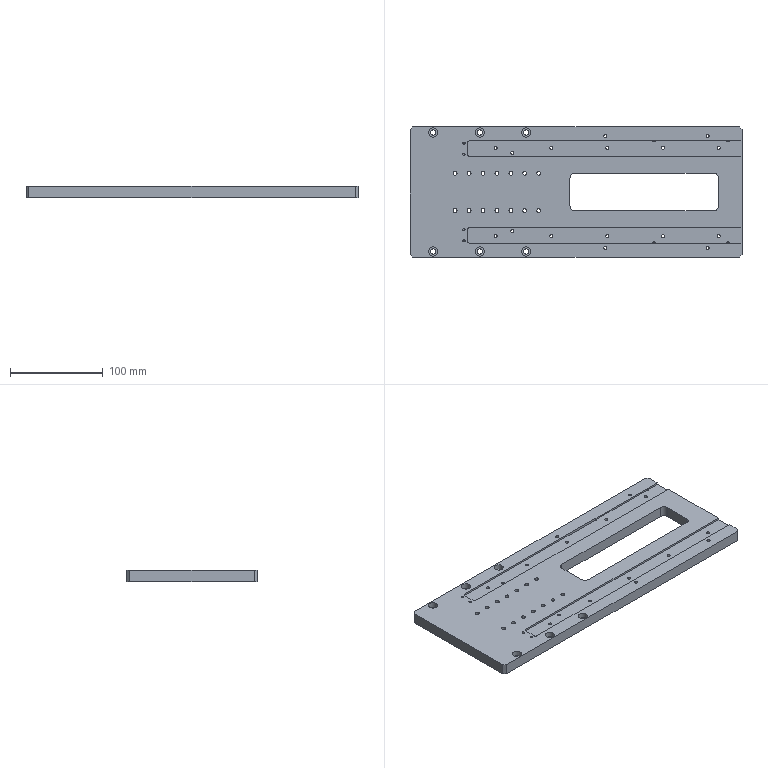NC program | NX | posted with a generic post | part box 357 x 140 x 12 mm
Whole program:
N10 G17 G21 G94 G90
(DRILLING_COPY , TOOL : D6A45)
N12 T01 M6
N14 G54
N16 G17 G0 G90 X-163.5 Y55. B0. C0. S9500 M3
N18 G43 Z30. H1
N20 G94 G81 G98 Z-1. F250. R3.
N22 X-83.8
N24 Y-55.
N26 X-163.5
N28 G80
N30 G0 X-163.5 Y-55. Z30.
N32 M5
(DRILLING_COPY_COPY_1 , TOOL : 2.5ZT)
N34 T02 M6
N36 G54
N38 G17 G0 G90 X-163.5 Y55. B0. C0. S1500 M3
N40 G43 Z30. H2
N42 G94 G83 G98 Z-10.601 F120. Q2. R3.
N44 X-83.8
N46 Y-55.
N48 X-163.5
N50 G80
N52 G0 X-163.5 Y-55. Z30.
N54 M5
(PLANAR_MILL_COPY_COPY , TOOL : D6A45)
N56 T01 M6
N58 G54
N60 G17 G0 G90 X-163.4 Y-55.217 B0. C0. S8500 M3
N62 G43 Z30. H1
N64 Z0.5
N66 G94 G1 Z-1. F1250.
N68 G3 X-163.85 Y-55. R0.5
N70 X-163.5 Y-55.35 R0.35
N72 X-163.85 Y-55. R-0.35
N74 X-163.4 Y-54.783 R0.5
N76 G1 Z0.5
N78 G0 Z30.
N80 X-153.933 Y-48.
N82 Z0.5
N84 G1 Z-1.
N86 G3 X-153.5 Y-48.25 R0.5
N88 X-152.75 Y-47.5 R0.75
N90 X-153.5 Y-48.25 R-0.75
N92 X-153.067 Y-48. R0.5
N94 G1 Z0.5
N96 G0 Z30.
N98 X-141.933 Y-60.5
N100 Z0.5
N102 G1 Z-1.
N104 G3 X-141.5 Y-60.75 R0.5
N106 X-140.75 Y-60. R0.75
N108 X-141.5 Y-60.75 R-0.75
N110 X-141.067 Y-60.5 R0.5
N112 G1 Z0.5
N114 G0 Z30.
N116 X-93.933 Y-48.
N118 Z0.5
N120 G1 Z-1.
N122 G3 X-93.5 Y-48.25 R0.5
N124 X-92.75 Y-47.5 R0.75
N126 X-93.5 Y-48.25 R-0.75
N128 X-93.067 Y-48. R0.5
N130 G1 Z0.5
N132 G0 Z30.
N134 X-83.547 Y-54.918
N136 Z0.5
N138 G1 Z-1.
N140 G3 X-83.8 Y-55.35 R0.5
N142 X-83.45 Y-55. R0.35
N144 X-83.8 Y-55.35 R-0.35
N146 X-83.98 Y-54.883 R0.5
N148 G1 Z0.5
N150 G0 Z30.
N152 X-31.933 Y-60.5
N154 Z0.5
N156 G1 Z-1.
N158 G3 X-31.5 Y-60.75 R0.5
N160 X-30.75 Y-60. R0.75
N162 X-31.5 Y-60.75 R-0.75
N164 X-31.067 Y-60.5 R0.5
N166 G1 Z0.5
N168 G0 Z30.
N170 X-33.933 Y-48.
N172 Z0.5
N174 G1 Z-1.
N176 G3 X-33.5 Y-48.25 R0.5
N178 X-32.75 Y-47.5 R0.75
N180 X-33.5 Y-48.25 R-0.75
N182 X-33.067 Y-48. R0.5
N184 G1 Z0.5
N186 G0 Z30.
N188 X-74.366 Y-18.6
N190 Z0.5
N192 G1 Z-1.
N194 G3 X-73.5 Y-19.1 R1.
N196 G1 X1.5
N198 G3 X5.6 Y-15. R4.1
N200 G1 Y15.
N202 G3 X1.5 Y19.1 R4.1
N204 G1 X-148.5
N206 G3 X-152.6 Y15. R4.1
N208 G1 Y-15.
N210 G3 X-148.5 Y-19.1 R4.1
N212 G1 X-73.5
N214 G3 X-72.634 Y-18.6 R1.
N216 G1 Z0.5
N218 G0 Z30.
N220 X-93.067 Y48.
N222 Z0.5
N224 G1 Z-1.
N226 G3 X-93.5 Y48.25 R0.5
N228 X-94.25 Y47.5 R0.75
N230 X-93.5 Y48.25 R-0.75
N232 X-93.933 Y48. R0.5
N234 G1 Z0.5
N236 G0 Z30.
N238 X-153.067
N240 Z0.5
N242 G1 Z-1.
N244 G3 X-153.5 Y48.25 R0.5
N246 X-154.25 Y47.5 R0.75
N248 X-153.5 Y48.25 R-0.75
N250 X-153.933 Y48. R0.5
N252 G1 Z0.5
N254 G0 Z30.
N256 X-163.4 Y54.783
N258 Z0.5
N260 G1 Z-1.
N262 G3 X-163.85 Y55. R0.5
N264 X-163.5 Y54.65 R0.35
N266 X-163.85 Y55. R-0.35
N268 X-163.4 Y55.217 R0.5
N270 G1 Z0.5
N272 G0 Z30.
N274 X-141.067 Y60.5
N276 Z0.5
N278 G1 Z-1.
N280 G3 X-141.5 Y60.75 R0.5
N282 X-142.25 Y60. R0.75
N284 X-141.5 Y60.75 R-0.75
N286 X-141.933 Y60.5 R0.5
N288 G1 Z0.5
N290 G0 Z30.
N292 X-83.98 Y54.883
N294 Z0.5
N296 G1 Z-1.
N298 G3 X-83.8 Y55.35 R0.5
N300 X-84.15 Y55. R0.35
N302 X-83.8 Y55.35 R-0.35
N304 X-83.547 Y54.919 R0.5
N306 G1 Z0.5
N308 G0 Z30.
N310 X-31.067 Y60.5
N312 Z0.5
N314 G1 Z-1.
N316 G3 X-31.5 Y60.75 R0.5
N318 X-32.25 Y60. R0.75
N320 X-31.5 Y60.75 R-0.75
N322 X-31.933 Y60.5 R0.5
N324 G1 Z0.5
N326 G0 Z30.
N328 X-33.067 Y48.
N330 Z0.5
N332 G1 Z-1.
N334 G3 X-33.5 Y48.25 R0.5
N336 X-34.25 Y47.5 R0.75
N338 X-33.5 Y48.25 R-0.75
N340 X-33.933 Y48. R0.5
N342 G1 Z0.5
N344 G0 Z30.
N346 X-0.866 Y71.4
N348 Z0.5
N350 G1 Z-1.
N352 G3 X0. Y70.9 R1.
N354 G1 X175.5
N356 G2 X176.136 Y70.636 R0.9
N358 G1 X179.136 Y67.636
N360 G2 X179.4 Y67. R0.9
N362 G1 Y-67.
N364 G2 X179.136 Y-67.636 R0.9
N366 G1 X176.136 Y-70.636
N368 G2 X175.5 Y-70.9 R0.9
N370 G1 X-175.5
N372 G2 X-176.136 Y-70.636 R0.9
N374 G1 X-179.136 Y-67.636
N376 G2 X-179.4 Y-67. R0.9
N378 G1 Y67.
N380 G2 X-179.136 Y67.636 R0.9
N382 G1 X-176.136 Y70.636
N384 G2 X-175.5 Y70.9 R0.9
N386 G1 X0.
N388 G3 X0.866 Y71.4 R1.
N390 G1 Z0.5
N392 G0 Z30.
N394 X40.866 Y20.7
N396 Z0.5
N398 G1 Z-1.
N400 G3 X40. Y21.2 R1.
N402 X38.8 Y20. R1.2
N404 X40. Y21.2 R-1.2
N406 X39.134 Y20.7 R1.
N408 G1 Z0.5
N410 G0 Z30.
N412 X26.933 Y48.
N414 Z0.5
N416 G1 Z-1.
N418 G3 X26.5 Y48.25 R0.5
N420 X25.75 Y47.5 R0.75
N422 X26.5 Y48.25 R-0.75
N424 X26.067 Y48. R0.5
N426 G1 Z0.5
N428 G0 Z30.
N430 X54.366 Y65.35
N432 Z0.5
N434 G1 Z-1.
N436 G3 X53.5 Y65.85 R1.
N438 X51.65 Y64. R1.85
N440 X53.5 Y65.85 R-1.85
N442 X52.634 Y65.35 R1.
N444 G1 Z0.5
N446 G0 Z30.
N448 X68.933 Y42.5
N450 Z0.5
N452 G1 Z-1.
N454 G3 X68.5 Y42.75 R0.5
N456 X67.75 Y42. R0.75
N458 X68.5 Y42.75 R-0.75
N460 X68.067 Y42.5 R0.5
N462 G1 Z0.5
N464 G0 Z30.
N466 X86.933 Y48.
N468 Z0.5
N470 G1 Z-1.
N472 G3 X86.5 Y48.25 R0.5
N474 X85.75 Y47.5 R0.75
N476 X86.5 Y48.25 R-0.75
N478 X86.067 Y48. R0.5
N480 G1 Z0.5
N482 G0 Z30.
N484 X104.366 Y65.35
N486 Z0.5
N488 G1 Z-1.
N490 G3 X103.5 Y65.85 R1.
N492 X101.65 Y64. R1.85
N494 X103.5 Y65.85 R-1.85
N496 X102.634 Y65.35 R1.
N498 G1 Z0.5
N500 G0 Z30.
N502 X154.366
N504 Z0.5
N506 G1 Z-1.
N508 G3 X153.5 Y65.85 R1.
N510 X151.65 Y64. R1.85
N512 X153.5 Y65.85 R-1.85
N514 X152.634 Y65.35 R1.
N516 G1 Z0.5
N518 G0 Z30.
N520 X130.7 Y19.134
N522 Z0.5
N524 G1 Z-1.
N526 G3 X131.2 Y20. R1.
N528 X130. Y21.2 R1.2
N530 X131.2 Y20. R-1.2
N532 X130.7 Y20.866 R1.
N534 G1 Z0.5
N536 G0 Z30.
N538 X115.866 Y20.7
N540 Z0.5
N542 G1 Z-1.
N544 G3 X115. Y21.2 R1.
N546 X113.8 Y20. R1.2
N548 X115. Y21.2 R-1.2
N550 X114.134 Y20.7 R1.
N552 G1 Z0.5
N554 G0 Z30.
N556 X100.866
N558 Z0.5
N560 G1 Z-1.
N562 G3 X100. Y21.2 R1.
N564 X98.8 Y20. R1.2
N566 X100. Y21.2 R-1.2
N568 X99.134 Y20.7 R1.
N570 G1 Z0.5
N572 G0 Z30.
N574 X85.866
N576 Z0.5
N578 G1 Z-1.
N580 G3 X85. Y21.2 R1.
N582 X83.8 Y20. R1.2
N584 X85. Y21.2 R-1.2
N586 X84.134 Y20.7 R1.
N588 G1 Z0.5
N590 G0 Z30.
N592 X70.866
N594 Z0.5
N596 G1 Z-1.
N598 G3 X70. Y21.2 R1.
N600 X68.8 Y20. R1.2
N602 X70. Y21.2 R-1.2
N604 X69.134 Y20.7 R1.
N606 G1 Z0.5
N608 G0 Z30.
N610 X55.866
N612 Z0.5
N614 G1 Z-1.
N616 G3 X55. Y21.2 R1.
N618 X53.8 Y20. R1.2
N620 X55. Y21.2 R-1.2
N622 X54.134 Y20.7 R1.
N624 G1 Z0.5
N626 G0 Z30.
N628 Y-20.7
N630 Z0.5
N632 G1 Z-1.
N634 G3 X55. Y-21.2 R1.
N636 X56.2 Y-20. R1.2
N638 X55. Y-21.2 R-1.2
N640 X55.866 Y-20.7 R1.
N642 G1 Z0.5
N644 G0 Z30.
N646 X39.134
N648 Z0.5
N650 G1 Z-1.
N652 G3 X40. Y-21.2 R1.
N654 X41.2 Y-20. R1.2
N656 X40. Y-21.2 R-1.2
N658 X40.866 Y-20.7 R1.
N660 G1 Z0.5
N662 G0 Z30.
N664 X26.067 Y-48.
N666 Z0.5
N668 G1 Z-1.
N670 G3 X26.5 Y-48.25 R0.5
N672 X27.25 Y-47.5 R0.75
N674 X26.5 Y-48.25 R-0.75
N676 X26.933 Y-48. R0.5
N678 G1 Z0.5
N680 G0 Z30.
N682 X52.634 Y-65.35
N684 Z0.5
N686 G1 Z-1.
N688 G3 X53.5 Y-65.85 R1.
N690 X55.35 Y-64. R1.85
N692 X53.5 Y-65.85 R-1.85
N694 X54.366 Y-65.35 R1.
N696 G1 Z0.5
N698 G0 Z30.
N700 X102.634
N702 Z0.5
N704 G1 Z-1.
N706 G3 X103.5 Y-65.85 R1.
N708 X105.35 Y-64. R1.85
N710 X103.5 Y-65.85 R-1.85
N712 X104.366 Y-65.35 R1.
N714 G1 Z0.5
N716 G0 Z30.
N718 X86.067 Y-48.
N720 Z0.5
N722 G1 Z-1.
N724 G3 X86.5 Y-48.25 R0.5
N726 X87.25 Y-47.5 R0.75
N728 X86.5 Y-48.25 R-0.75
N730 X86.933 Y-48. R0.5
N732 G1 Z0.5
N734 G0 Z30.
N736 X68.067 Y-42.5
N738 Z0.5
N740 G1 Z-1.
N742 G3 X68.5 Y-42.75 R0.5
N744 X69.25 Y-42. R0.75
N746 X68.5 Y-42.75 R-0.75
N748 X68.933 Y-42.5 R0.5
N750 G1 Z0.5
N752 G0 Z30.
N754 X69.134 Y-20.7
N756 Z0.5
N758 G1 Z-1.
N760 G3 X70. Y-21.2 R1.
N762 X71.2 Y-20. R1.2
N764 X70. Y-21.2 R-1.2
N766 X70.866 Y-20.7 R1.
N768 G1 Z0.5
N770 G0 Z30.
N772 X84.134
N774 Z0.5
N776 G1 Z-1.
N778 G3 X85. Y-21.2 R1.
N780 X86.2 Y-20. R1.2
N782 X85. Y-21.2 R-1.2
N784 X85.866 Y-20.7 R1.
N786 G1 Z0.5
N788 G0 Z30.
N790 X99.134
N792 Z0.5
N794 G1 Z-1.
N796 G3 X100. Y-21.2 R1.
N798 X101.2 Y-20. R1.2
N800 X100. Y-21.2 R-1.2
N802 X100.866 Y-20.7 R1.
N804 G1 Z0.5
N806 G0 Z30.
N808 X114.134
N810 Z0.5
N812 G1 Z-1.
N814 G3 X115. Y-21.2 R1.
N816 X116.2 Y-20. R1.2
N818 X115. Y-21.2 R-1.2
N820 X115.866 Y-20.7 R1.
N822 G1 Z0.5
N824 G0 Z30.
N826 X130.7 Y-20.866
N828 Z0.5
N830 G1 Z-1.
N832 G3 X131.2 Y-20. R1.
N834 X130. Y-18.8 R1.2
N836 X131.2 Y-20. R-1.2
N838 X130.7 Y-19.134 R1.
N840 G1 Z0.5
N842 G0 Z30.
N844 X152.634 Y-65.35
N846 Z0.5
N848 G1 Z-1.
N850 G3 X153.5 Y-65.85 R1.
N852 X155.35 Y-64. R1.85
N854 X153.5 Y-65.85 R-1.85
N856 X154.366 Y-65.35 R1.
N858 G1 Z0.5
N860 G0 Z30.
N862 M5
N864 M2